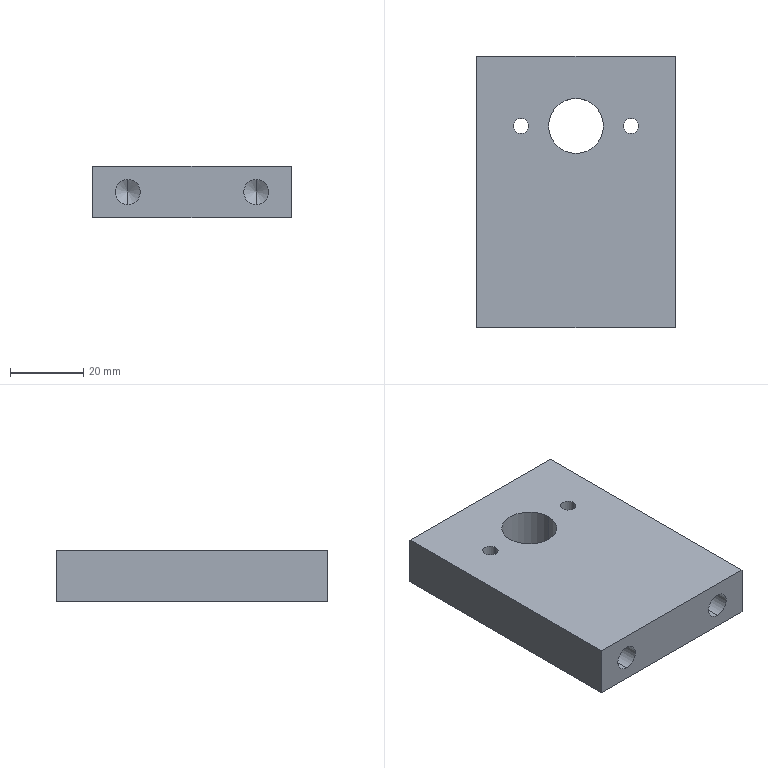Part | STEP file | PN_0065 (support block) | 1 solid | 20 faces | box 54 x 74 x 14 mm | volume 51598 mm3 | cylinder 10 | plane 6 | cone 4 | commonest cylinder face diameters 4.2 x4 6.8 x4 15 x2
STEP:
#1=CARTESIAN_POINT('',(0.,0.,0.));
#2=DIRECTION('',(0.,0.,1.));
#3=DIRECTION('',(1.,0.,0.));
#4=AXIS2_PLACEMENT_3D('',#1,#2,#3);
#5=CARTESIAN_POINT('',(-12.9,55.,-7.));
#6=VERTEX_POINT('',#5);
#7=CARTESIAN_POINT('',(-12.9,55.,7.));
#8=VERTEX_POINT('',#7);
#9=CARTESIAN_POINT('',(-12.9,55.,7.));
#10=DIRECTION('',(0.,0.,1.));
#11=VECTOR('',#10,1.);
#12=LINE('',#9,#11);
#13=CARTESIAN_POINT('',(-15.,55.,7.));
#14=DIRECTION('',(0.,0.,1.));
#15=DIRECTION('',(1.,0.,0.));
#16=AXIS2_PLACEMENT_3D('',#13,#14,#15);
#17=CYLINDRICAL_SURFACE('',#16,2.1);
#18=CARTESIAN_POINT('',(6.283,0.));
#19=DIRECTION('',(0.,1.));
#20=VECTOR('',#19,1.);
#21=LINE('',#18,#20);
#22=(GEOMETRIC_REPRESENTATION_CONTEXT(2)PARAMETRIC_REPRESENTATION_CONTEXT()REPRESENTATION_CONTEXT('',''));
#23=DEFINITIONAL_REPRESENTATION('',(#21),#22);
#24=PCURVE('',#17,#23);
#25=CARTESIAN_POINT('',(-15.,55.,7.));
#26=DIRECTION('',(0.,0.,1.));
#27=DIRECTION('',(1.,0.,0.));
#28=AXIS2_PLACEMENT_3D('',#25,#26,#27);
#29=CYLINDRICAL_SURFACE('',#28,2.1);
#30=CARTESIAN_POINT('',(0.,0.));
#31=DIRECTION('',(0.,1.));
#32=VECTOR('',#31,1.);
#33=LINE('',#30,#32);
#34=(GEOMETRIC_REPRESENTATION_CONTEXT(2)PARAMETRIC_REPRESENTATION_CONTEXT()REPRESENTATION_CONTEXT('',''));
#35=DEFINITIONAL_REPRESENTATION('',(#33),#34);
#36=PCURVE('',#29,#35);
#37=SURFACE_CURVE('',#12,(#24,#36),.PCURVE_S1.);
#38=EDGE_CURVE('',#6,#8,#37,.T.);
#39=ORIENTED_EDGE('',*,*,#38,.T.);
#40=CARTESIAN_POINT('',(-17.1,55.,7.));
#41=VERTEX_POINT('',#40);
#42=CARTESIAN_POINT('',(-15.,55.,7.));
#43=DIRECTION('',(0.,0.,1.));
#44=DIRECTION('',(1.,0.,0.));
#45=AXIS2_PLACEMENT_3D('',#42,#43,#44);
#46=CIRCLE('',#45,2.1);
#47=CARTESIAN_POINT('',(0.,0.));
#48=DIRECTION('',(1.,0.));
#49=VECTOR('',#48,1.);
#50=LINE('',#47,#49);
#51=(GEOMETRIC_REPRESENTATION_CONTEXT(2)PARAMETRIC_REPRESENTATION_CONTEXT()REPRESENTATION_CONTEXT('',''));
#52=DEFINITIONAL_REPRESENTATION('',(#50),#51);
#53=PCURVE('',#17,#52);
#54=CARTESIAN_POINT('',(0.,0.,7.));
#55=DIRECTION('',(0.,0.,-1.));
#56=DIRECTION('',(-1.,0.,0.));
#57=AXIS2_PLACEMENT_3D('',#54,#55,#56);
#58=PLANE('',#57);
#59=CARTESIAN_POINT('',(12.9,55.));
#60=CARTESIAN_POINT('',(12.9,58.637));
#61=CARTESIAN_POINT('',(16.05,56.819));
#62=CARTESIAN_POINT('',(19.2,55.));
#63=CARTESIAN_POINT('',(16.05,53.181));
#64=CARTESIAN_POINT('',(12.9,51.363));
#65=CARTESIAN_POINT('',(12.9,55.));
#66=(BOUNDED_CURVE()B_SPLINE_CURVE(2,(#59,#60,#61,#62,#63,#64,#65),.UNSPECIFIED.,.T.,.F.)B_SPLINE_CURVE_WITH_KNOTS((1,2,2,2,2,1),(-2.094,0.,2.094,4.189,6.283,8.378),.UNSPECIFIED.)CURVE()GEOMETRIC_REPRESENTATION_ITEM()RATIONAL_B_SPLINE_CURVE((1.,0.5,1.,0.5,1.,0.5,1.))REPRESENTATION_ITEM(''));
#67=(GEOMETRIC_REPRESENTATION_CONTEXT(2)PARAMETRIC_REPRESENTATION_CONTEXT()REPRESENTATION_CONTEXT('',''));
#68=DEFINITIONAL_REPRESENTATION('',(#66),#67);
#69=PCURVE('',#58,#68);
#70=SURFACE_CURVE('',#46,(#53,#69),.PCURVE_S1.);
#71=EDGE_CURVE('',#41,#8,#70,.T.);
#72=ORIENTED_EDGE('',*,*,#71,.F.);
#73=CARTESIAN_POINT('',(-17.1,55.,-7.));
#74=VERTEX_POINT('',#73);
#75=CARTESIAN_POINT('',(-17.1,55.,7.));
#76=DIRECTION('',(0.,0.,1.));
#77=VECTOR('',#76,1.);
#78=LINE('',#75,#77);
#79=CARTESIAN_POINT('',(3.142,0.));
#80=DIRECTION('',(0.,1.));
#81=VECTOR('',#80,1.);
#82=LINE('',#79,#81);
#83=(GEOMETRIC_REPRESENTATION_CONTEXT(2)PARAMETRIC_REPRESENTATION_CONTEXT()REPRESENTATION_CONTEXT('',''));
#84=DEFINITIONAL_REPRESENTATION('',(#82),#83);
#85=PCURVE('',#17,#84);
#86=CARTESIAN_POINT('',(3.142,0.));
#87=DIRECTION('',(0.,1.));
#88=VECTOR('',#87,1.);
#89=LINE('',#86,#88);
#90=(GEOMETRIC_REPRESENTATION_CONTEXT(2)PARAMETRIC_REPRESENTATION_CONTEXT()REPRESENTATION_CONTEXT('',''));
#91=DEFINITIONAL_REPRESENTATION('',(#89),#90);
#92=PCURVE('',#29,#91);
#93=SURFACE_CURVE('',#78,(#85,#92),.PCURVE_S1.);
#94=EDGE_CURVE('',#74,#41,#93,.T.);
#95=ORIENTED_EDGE('',*,*,#94,.F.);
#96=CARTESIAN_POINT('',(-15.,55.,-7.));
#97=DIRECTION('',(0.,0.,1.));
#98=DIRECTION('',(1.,0.,0.));
#99=AXIS2_PLACEMENT_3D('',#96,#97,#98);
#100=CIRCLE('',#99,2.1);
#101=CARTESIAN_POINT('',(0.,-14.));
#102=DIRECTION('',(1.,0.));
#103=VECTOR('',#102,1.);
#104=LINE('',#101,#103);
#105=(GEOMETRIC_REPRESENTATION_CONTEXT(2)PARAMETRIC_REPRESENTATION_CONTEXT()REPRESENTATION_CONTEXT('',''));
#106=DEFINITIONAL_REPRESENTATION('',(#104),#105);
#107=PCURVE('',#17,#106);
#108=CARTESIAN_POINT('',(0.,0.,-7.));
#109=DIRECTION('',(0.,0.,-1.));
#110=DIRECTION('',(-1.,0.,0.));
#111=AXIS2_PLACEMENT_3D('',#108,#109,#110);
#112=PLANE('',#111);
#113=CARTESIAN_POINT('',(12.9,55.));
#114=CARTESIAN_POINT('',(12.9,58.637));
#115=CARTESIAN_POINT('',(16.05,56.819));
#116=CARTESIAN_POINT('',(19.2,55.));
#117=CARTESIAN_POINT('',(16.05,53.181));
#118=CARTESIAN_POINT('',(12.9,51.363));
#119=CARTESIAN_POINT('',(12.9,55.));
#120=(BOUNDED_CURVE()B_SPLINE_CURVE(2,(#113,#114,#115,#116,#117,#118,#119),.UNSPECIFIED.,.T.,.F.)B_SPLINE_CURVE_WITH_KNOTS((1,2,2,2,2,1),(-2.094,0.,2.094,4.189,6.283,8.378),.UNSPECIFIED.)CURVE()GEOMETRIC_REPRESENTATION_ITEM()RATIONAL_B_SPLINE_CURVE((1.,0.5,1.,0.5,1.,0.5,1.))REPRESENTATION_ITEM(''));
#121=(GEOMETRIC_REPRESENTATION_CONTEXT(2)PARAMETRIC_REPRESENTATION_CONTEXT()REPRESENTATION_CONTEXT('',''));
#122=DEFINITIONAL_REPRESENTATION('',(#120),#121);
#123=PCURVE('',#112,#122);
#124=SURFACE_CURVE('',#100,(#107,#123),.PCURVE_S1.);
#125=EDGE_CURVE('',#74,#6,#124,.T.);
#126=ORIENTED_EDGE('',*,*,#125,.T.);
#127=EDGE_LOOP('',(#39,#72,#95,#126));
#128=FACE_BOUND('',#127,.F.);
#129=ADVANCED_FACE('',(#128),#17,.F.);
#130=CARTESIAN_POINT('',(17.1,55.,-7.));
#131=VERTEX_POINT('',#130);
#132=CARTESIAN_POINT('',(17.1,55.,7.));
#133=VERTEX_POINT('',#132);
#134=CARTESIAN_POINT('',(17.1,55.,7.));
#135=DIRECTION('',(0.,0.,1.));
#136=VECTOR('',#135,1.);
#137=LINE('',#134,#136);
#138=CARTESIAN_POINT('',(15.,55.,7.));
#139=DIRECTION('',(0.,0.,1.));
#140=DIRECTION('',(1.,0.,0.));
#141=AXIS2_PLACEMENT_3D('',#138,#139,#140);
#142=CYLINDRICAL_SURFACE('',#141,2.1);
#143=CARTESIAN_POINT('',(6.283,0.));
#144=DIRECTION('',(0.,1.));
#145=VECTOR('',#144,1.);
#146=LINE('',#143,#145);
#147=(GEOMETRIC_REPRESENTATION_CONTEXT(2)PARAMETRIC_REPRESENTATION_CONTEXT()REPRESENTATION_CONTEXT('',''));
#148=DEFINITIONAL_REPRESENTATION('',(#146),#147);
#149=PCURVE('',#142,#148);
#150=CARTESIAN_POINT('',(15.,55.,7.));
#151=DIRECTION('',(0.,0.,1.));
#152=DIRECTION('',(1.,0.,0.));
#153=AXIS2_PLACEMENT_3D('',#150,#151,#152);
#154=CYLINDRICAL_SURFACE('',#153,2.1);
#155=CARTESIAN_POINT('',(0.,0.));
#156=DIRECTION('',(0.,1.));
#157=VECTOR('',#156,1.);
#158=LINE('',#155,#157);
#159=(GEOMETRIC_REPRESENTATION_CONTEXT(2)PARAMETRIC_REPRESENTATION_CONTEXT()REPRESENTATION_CONTEXT('',''));
#160=DEFINITIONAL_REPRESENTATION('',(#158),#159);
#161=PCURVE('',#154,#160);
#162=SURFACE_CURVE('',#137,(#149,#161),.PCURVE_S1.);
#163=EDGE_CURVE('',#131,#133,#162,.T.);
#164=ORIENTED_EDGE('',*,*,#163,.T.);
#165=CARTESIAN_POINT('',(12.9,55.,7.));
#166=VERTEX_POINT('',#165);
#167=CARTESIAN_POINT('',(15.,55.,7.));
#168=DIRECTION('',(0.,0.,1.));
#169=DIRECTION('',(1.,0.,0.));
#170=AXIS2_PLACEMENT_3D('',#167,#168,#169);
#171=CIRCLE('',#170,2.1);
#172=CARTESIAN_POINT('',(0.,0.));
#173=DIRECTION('',(1.,0.));
#174=VECTOR('',#173,1.);
#175=LINE('',#172,#174);
#176=(GEOMETRIC_REPRESENTATION_CONTEXT(2)PARAMETRIC_REPRESENTATION_CONTEXT()REPRESENTATION_CONTEXT('',''));
#177=DEFINITIONAL_REPRESENTATION('',(#175),#176);
#178=PCURVE('',#142,#177);
#179=CARTESIAN_POINT('',(-17.1,55.));
#180=CARTESIAN_POINT('',(-17.1,58.637));
#181=CARTESIAN_POINT('',(-13.95,56.819));
#182=CARTESIAN_POINT('',(-10.8,55.));
#183=CARTESIAN_POINT('',(-13.95,53.181));
#184=CARTESIAN_POINT('',(-17.1,51.363));
#185=CARTESIAN_POINT('',(-17.1,55.));
#186=(BOUNDED_CURVE()B_SPLINE_CURVE(2,(#179,#180,#181,#182,#183,#184,#185),.UNSPECIFIED.,.T.,.F.)B_SPLINE_CURVE_WITH_KNOTS((1,2,2,2,2,1),(-2.094,0.,2.094,4.189,6.283,8.378),.UNSPECIFIED.)CURVE()GEOMETRIC_REPRESENTATION_ITEM()RATIONAL_B_SPLINE_CURVE((1.,0.5,1.,0.5,1.,0.5,1.))REPRESENTATION_ITEM(''));
#187=(GEOMETRIC_REPRESENTATION_CONTEXT(2)PARAMETRIC_REPRESENTATION_CONTEXT()REPRESENTATION_CONTEXT('',''));
#188=DEFINITIONAL_REPRESENTATION('',(#186),#187);
#189=PCURVE('',#58,#188);
#190=SURFACE_CURVE('',#171,(#178,#189),.PCURVE_S1.);
#191=EDGE_CURVE('',#166,#133,#190,.T.);
#192=ORIENTED_EDGE('',*,*,#191,.F.);
#193=CARTESIAN_POINT('',(12.9,55.,-7.));
#194=VERTEX_POINT('',#193);
#195=CARTESIAN_POINT('',(12.9,55.,7.));
#196=DIRECTION('',(0.,0.,1.));
#197=VECTOR('',#196,1.);
#198=LINE('',#195,#197);
#199=CARTESIAN_POINT('',(3.142,0.));
#200=DIRECTION('',(0.,1.));
#201=VECTOR('',#200,1.);
#202=LINE('',#199,#201);
#203=(GEOMETRIC_REPRESENTATION_CONTEXT(2)PARAMETRIC_REPRESENTATION_CONTEXT()REPRESENTATION_CONTEXT('',''));
#204=DEFINITIONAL_REPRESENTATION('',(#202),#203);
#205=PCURVE('',#142,#204);
#206=CARTESIAN_POINT('',(3.142,0.));
#207=DIRECTION('',(0.,1.));
#208=VECTOR('',#207,1.);
#209=LINE('',#206,#208);
#210=(GEOMETRIC_REPRESENTATION_CONTEXT(2)PARAMETRIC_REPRESENTATION_CONTEXT()REPRESENTATION_CONTEXT('',''));
#211=DEFINITIONAL_REPRESENTATION('',(#209),#210);
#212=PCURVE('',#154,#211);
#213=SURFACE_CURVE('',#198,(#205,#212),.PCURVE_S1.);
#214=EDGE_CURVE('',#194,#166,#213,.T.);
#215=ORIENTED_EDGE('',*,*,#214,.F.);
#216=CARTESIAN_POINT('',(15.,55.,-7.));
#217=DIRECTION('',(0.,0.,1.));
#218=DIRECTION('',(1.,0.,0.));
#219=AXIS2_PLACEMENT_3D('',#216,#217,#218);
#220=CIRCLE('',#219,2.1);
#221=CARTESIAN_POINT('',(0.,-14.));
#222=DIRECTION('',(1.,0.));
#223=VECTOR('',#222,1.);
#224=LINE('',#221,#223);
#225=(GEOMETRIC_REPRESENTATION_CONTEXT(2)PARAMETRIC_REPRESENTATION_CONTEXT()REPRESENTATION_CONTEXT('',''));
#226=DEFINITIONAL_REPRESENTATION('',(#224),#225);
#227=PCURVE('',#142,#226);
#228=CARTESIAN_POINT('',(-17.1,55.));
#229=CARTESIAN_POINT('',(-17.1,58.637));
#230=CARTESIAN_POINT('',(-13.95,56.819));
#231=CARTESIAN_POINT('',(-10.8,55.));
#232=CARTESIAN_POINT('',(-13.95,53.181));
#233=CARTESIAN_POINT('',(-17.1,51.363));
#234=CARTESIAN_POINT('',(-17.1,55.));
#235=(BOUNDED_CURVE()B_SPLINE_CURVE(2,(#228,#229,#230,#231,#232,#233,#234),.UNSPECIFIED.,.T.,.F.)B_SPLINE_CURVE_WITH_KNOTS((1,2,2,2,2,1),(-2.094,0.,2.094,4.189,6.283,8.378),.UNSPECIFIED.)CURVE()GEOMETRIC_REPRESENTATION_ITEM()RATIONAL_B_SPLINE_CURVE((1.,0.5,1.,0.5,1.,0.5,1.))REPRESENTATION_ITEM(''));
#236=(GEOMETRIC_REPRESENTATION_CONTEXT(2)PARAMETRIC_REPRESENTATION_CONTEXT()REPRESENTATION_CONTEXT('',''));
#237=DEFINITIONAL_REPRESENTATION('',(#235),#236);
#238=PCURVE('',#112,#237);
#239=SURFACE_CURVE('',#220,(#227,#238),.PCURVE_S1.);
#240=EDGE_CURVE('',#194,#131,#239,.T.);
#241=ORIENTED_EDGE('',*,*,#240,.T.);
#242=EDGE_LOOP('',(#164,#192,#215,#241));
#243=FACE_BOUND('',#242,.F.);
#244=ADVANCED_FACE('',(#243),#142,.F.);
#245=CARTESIAN_POINT('',(-7.5,55.,7.));
#246=VERTEX_POINT('',#245);
#247=CARTESIAN_POINT('',(-7.5,55.,-7.));
#248=VERTEX_POINT('',#247);
#249=CARTESIAN_POINT('',(-7.5,55.,7.));
#250=DIRECTION('',(0.,0.,-1.));
#251=VECTOR('',#250,1.);
#252=LINE('',#249,#251);
#253=CARTESIAN_POINT('',(0.,55.,7.));
#254=DIRECTION('',(0.,0.,-1.));
#255=DIRECTION('',(-1.,0.,0.));
#256=AXIS2_PLACEMENT_3D('',#253,#254,#255);
#257=CYLINDRICAL_SURFACE('',#256,7.5);
#258=CARTESIAN_POINT('',(6.283,0.));
#259=DIRECTION('',(0.,1.));
#260=VECTOR('',#259,1.);
#261=LINE('',#258,#260);
#262=(GEOMETRIC_REPRESENTATION_CONTEXT(2)PARAMETRIC_REPRESENTATION_CONTEXT()REPRESENTATION_CONTEXT('',''));
#263=DEFINITIONAL_REPRESENTATION('',(#261),#262);
#264=PCURVE('',#257,#263);
#265=CARTESIAN_POINT('',(0.,55.,7.));
#266=DIRECTION('',(0.,0.,-1.));
#267=DIRECTION('',(-1.,0.,0.));
#268=AXIS2_PLACEMENT_3D('',#265,#266,#267);
#269=CYLINDRICAL_SURFACE('',#268,7.5);
#270=CARTESIAN_POINT('',(0.,0.));
#271=DIRECTION('',(0.,1.));
#272=VECTOR('',#271,1.);
#273=LINE('',#270,#272);
#274=(GEOMETRIC_REPRESENTATION_CONTEXT(2)PARAMETRIC_REPRESENTATION_CONTEXT()REPRESENTATION_CONTEXT('',''));
#275=DEFINITIONAL_REPRESENTATION('',(#273),#274);
#276=PCURVE('',#269,#275);
#277=SURFACE_CURVE('',#252,(#264,#276),.PCURVE_S1.);
#278=EDGE_CURVE('',#246,#248,#277,.T.);
#279=ORIENTED_EDGE('',*,*,#278,.T.);
#280=CARTESIAN_POINT('',(7.5,55.,-7.));
#281=VERTEX_POINT('',#280);
#282=CARTESIAN_POINT('',(0.,55.,-7.));
#283=DIRECTION('',(0.,0.,-1.));
#284=DIRECTION('',(-1.,0.,0.));
#285=AXIS2_PLACEMENT_3D('',#282,#283,#284);
#286=CIRCLE('',#285,7.5);
#287=CARTESIAN_POINT('',(0.,14.));
#288=DIRECTION('',(1.,0.));
#289=VECTOR('',#288,1.);
#290=LINE('',#287,#289);
#291=(GEOMETRIC_REPRESENTATION_CONTEXT(2)PARAMETRIC_REPRESENTATION_CONTEXT()REPRESENTATION_CONTEXT('',''));
#292=DEFINITIONAL_REPRESENTATION('',(#290),#291);
#293=PCURVE('',#257,#292);
#294=CARTESIAN_POINT('',(0.,55.));
#295=DIRECTION('',(1.,0.));
#296=AXIS2_PLACEMENT_2D('',#294,#295);
#297=CIRCLE('',#296,7.5);
#298=(GEOMETRIC_REPRESENTATION_CONTEXT(2)PARAMETRIC_REPRESENTATION_CONTEXT()REPRESENTATION_CONTEXT('',''));
#299=DEFINITIONAL_REPRESENTATION('',(#297),#298);
#300=PCURVE('',#112,#299);
#301=SURFACE_CURVE('',#286,(#293,#300),.PCURVE_S1.);
#302=EDGE_CURVE('',#281,#248,#301,.T.);
#303=ORIENTED_EDGE('',*,*,#302,.F.);
#304=CARTESIAN_POINT('',(7.5,55.,7.));
#305=VERTEX_POINT('',#304);
#306=CARTESIAN_POINT('',(7.5,55.,7.));
#307=DIRECTION('',(0.,0.,-1.));
#308=VECTOR('',#307,1.);
#309=LINE('',#306,#308);
#310=CARTESIAN_POINT('',(3.142,0.));
#311=DIRECTION('',(0.,1.));
#312=VECTOR('',#311,1.);
#313=LINE('',#310,#312);
#314=(GEOMETRIC_REPRESENTATION_CONTEXT(2)PARAMETRIC_REPRESENTATION_CONTEXT()REPRESENTATION_CONTEXT('',''));
#315=DEFINITIONAL_REPRESENTATION('',(#313),#314);
#316=PCURVE('',#257,#315);
#317=CARTESIAN_POINT('',(3.142,0.));
#318=DIRECTION('',(0.,1.));
#319=VECTOR('',#318,1.);
#320=LINE('',#317,#319);
#321=(GEOMETRIC_REPRESENTATION_CONTEXT(2)PARAMETRIC_REPRESENTATION_CONTEXT()REPRESENTATION_CONTEXT('',''));
#322=DEFINITIONAL_REPRESENTATION('',(#320),#321);
#323=PCURVE('',#269,#322);
#324=SURFACE_CURVE('',#309,(#316,#323),.PCURVE_S1.);
#325=EDGE_CURVE('',#305,#281,#324,.T.);
#326=ORIENTED_EDGE('',*,*,#325,.F.);
#327=CARTESIAN_POINT('',(0.,55.,7.));
#328=DIRECTION('',(0.,0.,-1.));
#329=DIRECTION('',(-1.,0.,0.));
#330=AXIS2_PLACEMENT_3D('',#327,#328,#329);
#331=CIRCLE('',#330,7.5);
#332=CARTESIAN_POINT('',(0.,0.));
#333=DIRECTION('',(1.,0.));
#334=VECTOR('',#333,1.);
#335=LINE('',#332,#334);
#336=(GEOMETRIC_REPRESENTATION_CONTEXT(2)PARAMETRIC_REPRESENTATION_CONTEXT()REPRESENTATION_CONTEXT('',''));
#337=DEFINITIONAL_REPRESENTATION('',(#335),#336);
#338=PCURVE('',#257,#337);
#339=CARTESIAN_POINT('',(0.,55.));
#340=DIRECTION('',(1.,0.));
#341=AXIS2_PLACEMENT_2D('',#339,#340);
#342=CIRCLE('',#341,7.5);
#343=(GEOMETRIC_REPRESENTATION_CONTEXT(2)PARAMETRIC_REPRESENTATION_CONTEXT()REPRESENTATION_CONTEXT('',''));
#344=DEFINITIONAL_REPRESENTATION('',(#342),#343);
#345=PCURVE('',#58,#344);
#346=SURFACE_CURVE('',#331,(#338,#345),.PCURVE_S1.);
#347=EDGE_CURVE('',#305,#246,#346,.T.);
#348=ORIENTED_EDGE('',*,*,#347,.T.);
#349=EDGE_LOOP('',(#279,#303,#326,#348));
#350=FACE_BOUND('',#349,.F.);
#351=ADVANCED_FACE('',(#350),#257,.F.);
#352=CARTESIAN_POINT('',(-17.5,19.75,-3.4));
#353=VERTEX_POINT('',#352);
#354=CARTESIAN_POINT('',(-17.5,0.,-3.4));
#355=VERTEX_POINT('',#354);
#356=CARTESIAN_POINT('',(-17.5,0.,-3.4));
#357=DIRECTION('',(0.,-1.,0.));
#358=VECTOR('',#357,1.);
#359=LINE('',#356,#358);
#360=CARTESIAN_POINT('',(-17.5,0.,0.));
#361=DIRECTION('',(0.,-1.,0.));
#362=DIRECTION('',(0.,0.,-1.));
#363=AXIS2_PLACEMENT_3D('',#360,#361,#362);
#364=CYLINDRICAL_SURFACE('',#363,3.4);
#365=CARTESIAN_POINT('',(6.283,0.));
#366=DIRECTION('',(0.,1.));
#367=VECTOR('',#366,1.);
#368=LINE('',#365,#367);
#369=(GEOMETRIC_REPRESENTATION_CONTEXT(2)PARAMETRIC_REPRESENTATION_CONTEXT()REPRESENTATION_CONTEXT('',''));
#370=DEFINITIONAL_REPRESENTATION('',(#368),#369);
#371=PCURVE('',#364,#370);
#372=CARTESIAN_POINT('',(-17.5,0.,0.));
#373=DIRECTION('',(0.,-1.,0.));
#374=DIRECTION('',(0.,0.,-1.));
#375=AXIS2_PLACEMENT_3D('',#372,#373,#374);
#376=CYLINDRICAL_SURFACE('',#375,3.4);
#377=CARTESIAN_POINT('',(0.,0.));
#378=DIRECTION('',(0.,1.));
#379=VECTOR('',#378,1.);
#380=LINE('',#377,#379);
#381=(GEOMETRIC_REPRESENTATION_CONTEXT(2)PARAMETRIC_REPRESENTATION_CONTEXT()REPRESENTATION_CONTEXT('',''));
#382=DEFINITIONAL_REPRESENTATION('',(#380),#381);
#383=PCURVE('',#376,#382);
#384=SURFACE_CURVE('',#359,(#371,#383),.PCURVE_S1.);
#385=EDGE_CURVE('',#353,#355,#384,.T.);
#386=ORIENTED_EDGE('',*,*,#385,.T.);
#387=CARTESIAN_POINT('',(-17.5,0.,3.4));
#388=VERTEX_POINT('',#387);
#389=CARTESIAN_POINT('',(-17.5,0.,0.));
#390=DIRECTION('',(0.,-1.,0.));
#391=DIRECTION('',(0.,0.,-1.));
#392=AXIS2_PLACEMENT_3D('',#389,#390,#391);
#393=CIRCLE('',#392,3.4);
#394=CARTESIAN_POINT('',(0.,0.));
#395=DIRECTION('',(1.,0.));
#396=VECTOR('',#395,1.);
#397=LINE('',#394,#396);
#398=(GEOMETRIC_REPRESENTATION_CONTEXT(2)PARAMETRIC_REPRESENTATION_CONTEXT()REPRESENTATION_CONTEXT('',''));
#399=DEFINITIONAL_REPRESENTATION('',(#397),#398);
#400=PCURVE('',#364,#399);
#401=CARTESIAN_POINT('',(-27.,0.,7.));
#402=DIRECTION('',(0.,1.,0.));
#403=DIRECTION('',(0.,0.,1.));
#404=AXIS2_PLACEMENT_3D('',#401,#402,#403);
#405=PLANE('',#404);
#406=CARTESIAN_POINT('',(-10.4,9.5));
#407=CARTESIAN_POINT('',(-10.4,15.389));
#408=CARTESIAN_POINT('',(-5.3,12.444));
#409=CARTESIAN_POINT('',(-0.2,9.5));
#410=CARTESIAN_POINT('',(-5.3,6.556));
#411=CARTESIAN_POINT('',(-10.4,3.611));
#412=CARTESIAN_POINT('',(-10.4,9.5));
#413=(BOUNDED_CURVE()B_SPLINE_CURVE(2,(#406,#407,#408,#409,#410,#411,#412),.UNSPECIFIED.,.T.,.F.)B_SPLINE_CURVE_WITH_KNOTS((1,2,2,2,2,1),(-2.094,0.,2.094,4.189,6.283,8.378),.UNSPECIFIED.)CURVE()GEOMETRIC_REPRESENTATION_ITEM()RATIONAL_B_SPLINE_CURVE((1.,0.5,1.,0.5,1.,0.5,1.))REPRESENTATION_ITEM(''));
#414=(GEOMETRIC_REPRESENTATION_CONTEXT(2)PARAMETRIC_REPRESENTATION_CONTEXT()REPRESENTATION_CONTEXT('',''));
#415=DEFINITIONAL_REPRESENTATION('',(#413),#414);
#416=PCURVE('',#405,#415);
#417=SURFACE_CURVE('',#393,(#400,#416),.PCURVE_S1.);
#418=EDGE_CURVE('',#388,#355,#417,.T.);
#419=ORIENTED_EDGE('',*,*,#418,.F.);
#420=CARTESIAN_POINT('',(-17.5,19.75,3.4));
#421=VERTEX_POINT('',#420);
#422=CARTESIAN_POINT('',(-17.5,0.,3.4));
#423=DIRECTION('',(0.,-1.,0.));
#424=VECTOR('',#423,1.);
#425=LINE('',#422,#424);
#426=CARTESIAN_POINT('',(3.142,0.));
#427=DIRECTION('',(0.,1.));
#428=VECTOR('',#427,1.);
#429=LINE('',#426,#428);
#430=(GEOMETRIC_REPRESENTATION_CONTEXT(2)PARAMETRIC_REPRESENTATION_CONTEXT()REPRESENTATION_CONTEXT('',''));
#431=DEFINITIONAL_REPRESENTATION('',(#429),#430);
#432=PCURVE('',#364,#431);
#433=CARTESIAN_POINT('',(3.142,0.));
#434=DIRECTION('',(0.,1.));
#435=VECTOR('',#434,1.);
#436=LINE('',#433,#435);
#437=(GEOMETRIC_REPRESENTATION_CONTEXT(2)PARAMETRIC_REPRESENTATION_CONTEXT()REPRESENTATION_CONTEXT('',''));
#438=DEFINITIONAL_REPRESENTATION('',(#436),#437);
#439=PCURVE('',#376,#438);
#440=SURFACE_CURVE('',#425,(#432,#439),.PCURVE_S1.);
#441=EDGE_CURVE('',#421,#388,#440,.T.);
#442=ORIENTED_EDGE('',*,*,#441,.F.);
#443=CARTESIAN_POINT('',(-17.5,19.75,0.));
#444=DIRECTION('',(0.,-1.,0.));
#445=DIRECTION('',(0.,0.,-1.));
#446=AXIS2_PLACEMENT_3D('',#443,#444,#445);
#447=CIRCLE('',#446,3.4);
#448=CARTESIAN_POINT('',(0.,-19.75));
#449=DIRECTION('',(1.,0.));
#450=VECTOR('',#449,1.);
#451=LINE('',#448,#450);
#452=(GEOMETRIC_REPRESENTATION_CONTEXT(2)PARAMETRIC_REPRESENTATION_CONTEXT()REPRESENTATION_CONTEXT('',''));
#453=DEFINITIONAL_REPRESENTATION('',(#451),#452);
#454=PCURVE('',#364,#453);
#455=CARTESIAN_POINT('',(-17.5,19.75,0.));
#456=DIRECTION('',(0.,-1.,0.));
#457=DIRECTION('',(0.,0.,-1.));
#458=AXIS2_PLACEMENT_3D('',#455,#456,#457);
#459=CONICAL_SURFACE('',#458,3.4,1.03);
#460=CARTESIAN_POINT('',(0.,0.));
#461=DIRECTION('',(1.,0.));
#462=VECTOR('',#461,1.);
#463=LINE('',#460,#462);
#464=(GEOMETRIC_REPRESENTATION_CONTEXT(2)PARAMETRIC_REPRESENTATION_CONTEXT()REPRESENTATION_CONTEXT('',''));
#465=DEFINITIONAL_REPRESENTATION('',(#463),#464);
#466=PCURVE('',#459,#465);
#467=SURFACE_CURVE('',#447,(#454,#466),.PCURVE_S1.);
#468=EDGE_CURVE('',#421,#353,#467,.T.);
#469=ORIENTED_EDGE('',*,*,#468,.T.);
#470=EDGE_LOOP('',(#386,#419,#442,#469));
#471=FACE_BOUND('',#470,.F.);
#472=ADVANCED_FACE('',(#471),#364,.F.);
#473=ORIENTED_EDGE('',*,*,#468,.F.);
#474=CARTESIAN_POINT('',(-17.5,21.793,0.));
#475=VERTEX_POINT('',#474);
#476=CARTESIAN_POINT('',(-17.5,19.75,3.4));
#477=DIRECTION('',(0.,-0.515,0.8572));
#478=VECTOR('',#477,1.);
#479=LINE('',#476,#478);
#480=CARTESIAN_POINT('',(3.142,0.));
#481=DIRECTION('',(0.,1.));
#482=VECTOR('',#481,1.);
#483=LINE('',#480,#482);
#484=(GEOMETRIC_REPRESENTATION_CONTEXT(2)PARAMETRIC_REPRESENTATION_CONTEXT()REPRESENTATION_CONTEXT('',''));
#485=DEFINITIONAL_REPRESENTATION('',(#483),#484);
#486=PCURVE('',#459,#485);
#487=CARTESIAN_POINT('',(-17.5,19.75,0.));
#488=DIRECTION('',(0.,-1.,0.));
#489=DIRECTION('',(0.,0.,-1.));
#490=AXIS2_PLACEMENT_3D('',#487,#488,#489);
#491=CONICAL_SURFACE('',#490,3.4,1.03);
#492=CARTESIAN_POINT('',(3.142,0.));
#493=DIRECTION('',(0.,1.));
#494=VECTOR('',#493,1.);
#495=LINE('',#492,#494);
#496=(GEOMETRIC_REPRESENTATION_CONTEXT(2)PARAMETRIC_REPRESENTATION_CONTEXT()REPRESENTATION_CONTEXT('',''));
#497=DEFINITIONAL_REPRESENTATION('',(#495),#496);
#498=PCURVE('',#491,#497);
#499=SURFACE_CURVE('',#479,(#486,#498),.PCURVE_S1.);
#500=EDGE_CURVE('',#475,#421,#499,.T.);
#501=ORIENTED_EDGE('',*,*,#500,.F.);
#502=CARTESIAN_POINT('',(-17.5,19.75,-3.4));
#503=DIRECTION('',(0.,-0.515,-0.8572));
#504=VECTOR('',#503,1.);
#505=LINE('',#502,#504);
#506=CARTESIAN_POINT('',(6.283,0.));
#507=DIRECTION('',(0.,1.));
#508=VECTOR('',#507,1.);
#509=LINE('',#506,#508);
#510=(GEOMETRIC_REPRESENTATION_CONTEXT(2)PARAMETRIC_REPRESENTATION_CONTEXT()REPRESENTATION_CONTEXT('',''));
#511=DEFINITIONAL_REPRESENTATION('',(#509),#510);
#512=PCURVE('',#459,#511);
#513=CARTESIAN_POINT('',(0.,0.));
#514=DIRECTION('',(0.,1.));
#515=VECTOR('',#514,1.);
#516=LINE('',#513,#515);
#517=(GEOMETRIC_REPRESENTATION_CONTEXT(2)PARAMETRIC_REPRESENTATION_CONTEXT()REPRESENTATION_CONTEXT('',''));
#518=DEFINITIONAL_REPRESENTATION('',(#516),#517);
#519=PCURVE('',#491,#518);
#520=SURFACE_CURVE('',#505,(#512,#519),.PCURVE_S1.);
#521=EDGE_CURVE('',#475,#353,#520,.T.);
#522=ORIENTED_EDGE('',*,*,#521,.T.);
#523=EDGE_LOOP('',(#473,#501,#522));
#524=FACE_BOUND('',#523,.F.);
#525=ADVANCED_FACE('',(#524),#459,.F.);
#526=CARTESIAN_POINT('',(17.5,19.75,-3.4));
#527=VERTEX_POINT('',#526);
#528=CARTESIAN_POINT('',(17.5,0.,-3.4));
#529=VERTEX_POINT('',#528);
#530=CARTESIAN_POINT('',(17.5,0.,-3.4));
#531=DIRECTION('',(0.,-1.,0.));
#532=VECTOR('',#531,1.);
#533=LINE('',#530,#532);
#534=CARTESIAN_POINT('',(17.5,0.,0.));
#535=DIRECTION('',(0.,-1.,0.));
#536=DIRECTION('',(0.,0.,-1.));
#537=AXIS2_PLACEMENT_3D('',#534,#535,#536);
#538=CYLINDRICAL_SURFACE('',#537,3.4);
#539=CARTESIAN_POINT('',(6.283,0.));
#540=DIRECTION('',(0.,1.));
#541=VECTOR('',#540,1.);
#542=LINE('',#539,#541);
#543=(GEOMETRIC_REPRESENTATION_CONTEXT(2)PARAMETRIC_REPRESENTATION_CONTEXT()REPRESENTATION_CONTEXT('',''));
#544=DEFINITIONAL_REPRESENTATION('',(#542),#543);
#545=PCURVE('',#538,#544);
#546=CARTESIAN_POINT('',(17.5,0.,0.));
#547=DIRECTION('',(0.,-1.,0.));
#548=DIRECTION('',(0.,0.,-1.));
#549=AXIS2_PLACEMENT_3D('',#546,#547,#548);
#550=CYLINDRICAL_SURFACE('',#549,3.4);
#551=CARTESIAN_POINT('',(0.,0.));
#552=DIRECTION('',(0.,1.));
#553=VECTOR('',#552,1.);
#554=LINE('',#551,#553);
#555=(GEOMETRIC_REPRESENTATION_CONTEXT(2)PARAMETRIC_REPRESENTATION_CONTEXT()REPRESENTATION_CONTEXT('',''));
#556=DEFINITIONAL_REPRESENTATION('',(#554),#555);
#557=PCURVE('',#550,#556);
#558=SURFACE_CURVE('',#533,(#545,#557),.PCURVE_S1.);
#559=EDGE_CURVE('',#527,#529,#558,.T.);
#560=ORIENTED_EDGE('',*,*,#559,.T.);
#561=CARTESIAN_POINT('',(17.5,0.,3.4));
#562=VERTEX_POINT('',#561);
#563=CARTESIAN_POINT('',(17.5,0.,0.));
#564=DIRECTION('',(0.,-1.,0.));
#565=DIRECTION('',(0.,0.,-1.));
#566=AXIS2_PLACEMENT_3D('',#563,#564,#565);
#567=CIRCLE('',#566,3.4);
#568=CARTESIAN_POINT('',(0.,0.));
#569=DIRECTION('',(1.,0.));
#570=VECTOR('',#569,1.);
#571=LINE('',#568,#570);
#572=(GEOMETRIC_REPRESENTATION_CONTEXT(2)PARAMETRIC_REPRESENTATION_CONTEXT()REPRESENTATION_CONTEXT('',''));
#573=DEFINITIONAL_REPRESENTATION('',(#571),#572);
#574=PCURVE('',#538,#573);
#575=CARTESIAN_POINT('',(-10.4,44.5));
#576=CARTESIAN_POINT('',(-10.4,50.389));
#577=CARTESIAN_POINT('',(-5.3,47.444));
#578=CARTESIAN_POINT('',(-0.2,44.5));
#579=CARTESIAN_POINT('',(-5.3,41.556));
#580=CARTESIAN_POINT('',(-10.4,38.611));
#581=CARTESIAN_POINT('',(-10.4,44.5));
#582=(BOUNDED_CURVE()B_SPLINE_CURVE(2,(#575,#576,#577,#578,#579,#580,#581),.UNSPECIFIED.,.T.,.F.)B_SPLINE_CURVE_WITH_KNOTS((1,2,2,2,2,1),(-2.094,0.,2.094,4.189,6.283,8.378),.UNSPECIFIED.)CURVE()GEOMETRIC_REPRESENTATION_ITEM()RATIONAL_B_SPLINE_CURVE((1.,0.5,1.,0.5,1.,0.5,1.))REPRESENTATION_ITEM(''));
#583=(GEOMETRIC_REPRESENTATION_CONTEXT(2)PARAMETRIC_REPRESENTATION_CONTEXT()REPRESENTATION_CONTEXT('',''));
#584=DEFINITIONAL_REPRESENTATION('',(#582),#583);
#585=PCURVE('',#405,#584);
#586=SURFACE_CURVE('',#567,(#574,#585),.PCURVE_S1.);
#587=EDGE_CURVE('',#562,#529,#586,.T.);
#588=ORIENTED_EDGE('',*,*,#587,.F.);
#589=CARTESIAN_POINT('',(17.5,19.75,3.4));
#590=VERTEX_POINT('',#589);
#591=CARTESIAN_POINT('',(17.5,0.,3.4));
#592=DIRECTION('',(0.,-1.,0.));
#593=VECTOR('',#592,1.);
#594=LINE('',#591,#593);
#595=CARTESIAN_POINT('',(3.142,0.));
#596=DIRECTION('',(0.,1.));
#597=VECTOR('',#596,1.);
#598=LINE('',#595,#597);
#599=(GEOMETRIC_REPRESENTATION_CONTEXT(2)PARAMETRIC_REPRESENTATION_CONTEXT()REPRESENTATION_CONTEXT('',''));
#600=DEFINITIONAL_REPRESENTATION('',(#598),#599);
#601=PCURVE('',#538,#600);
#602=CARTESIAN_POINT('',(3.142,0.));
#603=DIRECTION('',(0.,1.));
#604=VECTOR('',#603,1.);
#605=LINE('',#602,#604);
#606=(GEOMETRIC_REPRESENTATION_CONTEXT(2)PARAMETRIC_REPRESENTATION_CONTEXT()REPRESENTATION_CONTEXT('',''));
#607=DEFINITIONAL_REPRESENTATION('',(#605),#606);
#608=PCURVE('',#550,#607);
#609=SURFACE_CURVE('',#594,(#601,#608),.PCURVE_S1.);
#610=EDGE_CURVE('',#590,#562,#609,.T.);
#611=ORIENTED_EDGE('',*,*,#610,.F.);
#612=CARTESIAN_POINT('',(17.5,19.75,0.));
#613=DIRECTION('',(0.,-1.,0.));
#614=DIRECTION('',(0.,0.,-1.));
#615=AXIS2_PLACEMENT_3D('',#612,#613,#614);
#616=CIRCLE('',#615,3.4);
#617=CARTESIAN_POINT('',(0.,-19.75));
#618=DIRECTION('',(1.,0.));
#619=VECTOR('',#618,1.);
#620=LINE('',#617,#619);
#621=(GEOMETRIC_REPRESENTATION_CONTEXT(2)PARAMETRIC_REPRESENTATION_CONTEXT()REPRESENTATION_CONTEXT('',''));
#622=DEFINITIONAL_REPRESENTATION('',(#620),#621);
#623=PCURVE('',#538,#622);
#624=CARTESIAN_POINT('',(17.5,19.75,0.));
#625=DIRECTION('',(0.,-1.,0.));
#626=DIRECTION('',(0.,0.,-1.));
#627=AXIS2_PLACEMENT_3D('',#624,#625,#626);
#628=CONICAL_SURFACE('',#627,3.4,1.03);
#629=CARTESIAN_POINT('',(0.,0.));
#630=DIRECTION('',(1.,0.));
#631=VECTOR('',#630,1.);
#632=LINE('',#629,#631);
#633=(GEOMETRIC_REPRESENTATION_CONTEXT(2)PARAMETRIC_REPRESENTATION_CONTEXT()REPRESENTATION_CONTEXT('',''));
#634=DEFINITIONAL_REPRESENTATION('',(#632),#633);
#635=PCURVE('',#628,#634);
#636=SURFACE_CURVE('',#616,(#623,#635),.PCURVE_S1.);
#637=EDGE_CURVE('',#590,#527,#636,.T.);
#638=ORIENTED_EDGE('',*,*,#637,.T.);
#639=EDGE_LOOP('',(#560,#588,#611,#638));
#640=FACE_BOUND('',#639,.F.);
#641=ADVANCED_FACE('',(#640),#538,.F.);
#642=ORIENTED_EDGE('',*,*,#637,.F.);
#643=CARTESIAN_POINT('',(17.5,21.793,0.));
#644=VERTEX_POINT('',#643);
#645=CARTESIAN_POINT('',(17.5,19.75,3.4));
#646=DIRECTION('',(0.,-0.515,0.8572));
#647=VECTOR('',#646,1.);
#648=LINE('',#645,#647);
#649=CARTESIAN_POINT('',(3.142,0.));
#650=DIRECTION('',(0.,1.));
#651=VECTOR('',#650,1.);
#652=LINE('',#649,#651);
#653=(GEOMETRIC_REPRESENTATION_CONTEXT(2)PARAMETRIC_REPRESENTATION_CONTEXT()REPRESENTATION_CONTEXT('',''));
#654=DEFINITIONAL_REPRESENTATION('',(#652),#653);
#655=PCURVE('',#628,#654);
#656=CARTESIAN_POINT('',(17.5,19.75,0.));
#657=DIRECTION('',(0.,-1.,0.));
#658=DIRECTION('',(0.,0.,-1.));
#659=AXIS2_PLACEMENT_3D('',#656,#657,#658);
#660=CONICAL_SURFACE('',#659,3.4,1.03);
#661=CARTESIAN_POINT('',(3.142,0.));
#662=DIRECTION('',(0.,1.));
#663=VECTOR('',#662,1.);
#664=LINE('',#661,#663);
#665=(GEOMETRIC_REPRESENTATION_CONTEXT(2)PARAMETRIC_REPRESENTATION_CONTEXT()REPRESENTATION_CONTEXT('',''));
#666=DEFINITIONAL_REPRESENTATION('',(#664),#665);
#667=PCURVE('',#660,#666);
#668=SURFACE_CURVE('',#648,(#655,#667),.PCURVE_S1.);
#669=EDGE_CURVE('',#644,#590,#668,.T.);
#670=ORIENTED_EDGE('',*,*,#669,.F.);
#671=CARTESIAN_POINT('',(17.5,19.75,-3.4));
#672=DIRECTION('',(0.,-0.515,-0.8572));
#673=VECTOR('',#672,1.);
#674=LINE('',#671,#673);
#675=CARTESIAN_POINT('',(6.283,0.));
#676=DIRECTION('',(0.,1.));
#677=VECTOR('',#676,1.);
#678=LINE('',#675,#677);
#679=(GEOMETRIC_REPRESENTATION_CONTEXT(2)PARAMETRIC_REPRESENTATION_CONTEXT()REPRESENTATION_CONTEXT('',''));
#680=DEFINITIONAL_REPRESENTATION('',(#678),#679);
#681=PCURVE('',#628,#680);
#682=CARTESIAN_POINT('',(0.,0.));
#683=DIRECTION('',(0.,1.));
#684=VECTOR('',#683,1.);
#685=LINE('',#682,#684);
#686=(GEOMETRIC_REPRESENTATION_CONTEXT(2)PARAMETRIC_REPRESENTATION_CONTEXT()REPRESENTATION_CONTEXT('',''));
#687=DEFINITIONAL_REPRESENTATION('',(#685),#686);
#688=PCURVE('',#660,#687);
#689=SURFACE_CURVE('',#674,(#681,#688),.PCURVE_S1.);
#690=EDGE_CURVE('',#644,#527,#689,.T.);
#691=ORIENTED_EDGE('',*,*,#690,.T.);
#692=EDGE_LOOP('',(#642,#670,#691));
#693=FACE_BOUND('',#692,.F.);
#694=ADVANCED_FACE('',(#693),#628,.F.);
#695=CARTESIAN_POINT('',(-27.,74.,-7.));
#696=VERTEX_POINT('',#695);
#697=CARTESIAN_POINT('',(-27.,0.,-7.));
#698=VERTEX_POINT('',#697);
#699=CARTESIAN_POINT('',(-27.,0.,-7.));
#700=DIRECTION('',(0.,-1.,0.));
#701=VECTOR('',#700,1.);
#702=LINE('',#699,#701);
#703=CARTESIAN_POINT('',(-27.,0.,7.));
#704=DIRECTION('',(1.,0.,0.));
#705=DIRECTION('',(0.,0.,-1.));
#706=AXIS2_PLACEMENT_3D('',#703,#704,#705);
#707=PLANE('',#706);
#708=CARTESIAN_POINT('',(14.,0.));
#709=DIRECTION('',(0.,-1.));
#710=VECTOR('',#709,1.);
#711=LINE('',#708,#710);
#712=(GEOMETRIC_REPRESENTATION_CONTEXT(2)PARAMETRIC_REPRESENTATION_CONTEXT()REPRESENTATION_CONTEXT('',''));
#713=DEFINITIONAL_REPRESENTATION('',(#711),#712);
#714=PCURVE('',#707,#713);
#715=CARTESIAN_POINT('',(27.,0.));
#716=DIRECTION('',(0.,-1.));
#717=VECTOR('',#716,1.);
#718=LINE('',#715,#717);
#719=(GEOMETRIC_REPRESENTATION_CONTEXT(2)PARAMETRIC_REPRESENTATION_CONTEXT()REPRESENTATION_CONTEXT('',''));
#720=DEFINITIONAL_REPRESENTATION('',(#718),#719);
#721=PCURVE('',#112,#720);
#722=SURFACE_CURVE('',#702,(#714,#721),.PCURVE_S1.);
#723=EDGE_CURVE('',#696,#698,#722,.T.);
#724=ORIENTED_EDGE('',*,*,#723,.T.);
#725=CARTESIAN_POINT('',(-27.,0.,7.));
#726=VERTEX_POINT('',#725);
#727=CARTESIAN_POINT('',(-27.,0.,7.));
#728=DIRECTION('',(0.,0.,-1.));
#729=VECTOR('',#728,1.);
#730=LINE('',#727,#729);
#731=CARTESIAN_POINT('',(0.,0.));
#732=DIRECTION('',(1.,0.));
#733=VECTOR('',#732,1.);
#734=LINE('',#731,#733);
#735=(GEOMETRIC_REPRESENTATION_CONTEXT(2)PARAMETRIC_REPRESENTATION_CONTEXT()REPRESENTATION_CONTEXT('',''));
#736=DEFINITIONAL_REPRESENTATION('',(#734),#735);
#737=PCURVE('',#707,#736);
#738=CARTESIAN_POINT('',(0.,0.));
#739=DIRECTION('',(-1.,0.));
#740=VECTOR('',#739,1.);
#741=LINE('',#738,#740);
#742=(GEOMETRIC_REPRESENTATION_CONTEXT(2)PARAMETRIC_REPRESENTATION_CONTEXT()REPRESENTATION_CONTEXT('',''));
#743=DEFINITIONAL_REPRESENTATION('',(#741),#742);
#744=PCURVE('',#405,#743);
#745=SURFACE_CURVE('',#730,(#737,#744),.PCURVE_S1.);
#746=EDGE_CURVE('',#726,#698,#745,.T.);
#747=ORIENTED_EDGE('',*,*,#746,.F.);
#748=CARTESIAN_POINT('',(-27.,74.,7.));
#749=VERTEX_POINT('',#748);
#750=CARTESIAN_POINT('',(-27.,0.,7.));
#751=DIRECTION('',(0.,-1.,0.));
#752=VECTOR('',#751,1.);
#753=LINE('',#750,#752);
#754=CARTESIAN_POINT('',(0.,0.));
#755=DIRECTION('',(0.,-1.));
#756=VECTOR('',#755,1.);
#757=LINE('',#754,#756);
#758=(GEOMETRIC_REPRESENTATION_CONTEXT(2)PARAMETRIC_REPRESENTATION_CONTEXT()REPRESENTATION_CONTEXT('',''));
#759=DEFINITIONAL_REPRESENTATION('',(#757),#758);
#760=PCURVE('',#707,#759);
#761=CARTESIAN_POINT('',(27.,0.));
#762=DIRECTION('',(0.,-1.));
#763=VECTOR('',#762,1.);
#764=LINE('',#761,#763);
#765=(GEOMETRIC_REPRESENTATION_CONTEXT(2)PARAMETRIC_REPRESENTATION_CONTEXT()REPRESENTATION_CONTEXT('',''));
#766=DEFINITIONAL_REPRESENTATION('',(#764),#765);
#767=PCURVE('',#58,#766);
#768=SURFACE_CURVE('',#753,(#760,#767),.PCURVE_S1.);
#769=EDGE_CURVE('',#749,#726,#768,.T.);
#770=ORIENTED_EDGE('',*,*,#769,.F.);
#771=CARTESIAN_POINT('',(-27.,74.,7.));
#772=DIRECTION('',(0.,0.,-1.));
#773=VECTOR('',#772,1.);
#774=LINE('',#771,#773);
#775=CARTESIAN_POINT('',(0.,74.));
#776=DIRECTION('',(1.,0.));
#777=VECTOR('',#776,1.);
#778=LINE('',#775,#777);
#779=(GEOMETRIC_REPRESENTATION_CONTEXT(2)PARAMETRIC_REPRESENTATION_CONTEXT()REPRESENTATION_CONTEXT('',''));
#780=DEFINITIONAL_REPRESENTATION('',(#778),#779);
#781=PCURVE('',#707,#780);
#782=CARTESIAN_POINT('',(-27.,74.,7.));
#783=DIRECTION('',(0.,-1.,0.));
#784=DIRECTION('',(0.,0.,-1.));
#785=AXIS2_PLACEMENT_3D('',#782,#783,#784);
#786=PLANE('',#785);
#787=CARTESIAN_POINT('',(0.,0.));
#788=DIRECTION('',(1.,0.));
#789=VECTOR('',#788,1.);
#790=LINE('',#787,#789);
#791=(GEOMETRIC_REPRESENTATION_CONTEXT(2)PARAMETRIC_REPRESENTATION_CONTEXT()REPRESENTATION_CONTEXT('',''));
#792=DEFINITIONAL_REPRESENTATION('',(#790),#791);
#793=PCURVE('',#786,#792);
#794=SURFACE_CURVE('',#774,(#781,#793),.PCURVE_S1.);
#795=EDGE_CURVE('',#749,#696,#794,.T.);
#796=ORIENTED_EDGE('',*,*,#795,.T.);
#797=EDGE_LOOP('',(#724,#747,#770,#796));
#798=FACE_BOUND('',#797,.T.);
#799=ADVANCED_FACE('',(#798),#707,.F.);
#800=CARTESIAN_POINT('',(-17.5,0.,0.));
#801=DIRECTION('',(0.,-1.,0.));
#802=DIRECTION('',(0.,0.,-1.));
#803=AXIS2_PLACEMENT_3D('',#800,#801,#802);
#804=CIRCLE('',#803,3.4);
#805=CARTESIAN_POINT('',(-10.4,9.5));
#806=CARTESIAN_POINT('',(-10.4,15.389));
#807=CARTESIAN_POINT('',(-5.3,12.444));
#808=CARTESIAN_POINT('',(-0.2,9.5));
#809=CARTESIAN_POINT('',(-5.3,6.556));
#810=CARTESIAN_POINT('',(-10.4,3.611));
#811=CARTESIAN_POINT('',(-10.4,9.5));
#812=(BOUNDED_CURVE()B_SPLINE_CURVE(2,(#805,#806,#807,#808,#809,#810,#811),.UNSPECIFIED.,.T.,.F.)B_SPLINE_CURVE_WITH_KNOTS((1,2,2,2,2,1),(-2.094,0.,2.094,4.189,6.283,8.378),.UNSPECIFIED.)CURVE()GEOMETRIC_REPRESENTATION_ITEM()RATIONAL_B_SPLINE_CURVE((1.,0.5,1.,0.5,1.,0.5,1.))REPRESENTATION_ITEM(''));
#813=(GEOMETRIC_REPRESENTATION_CONTEXT(2)PARAMETRIC_REPRESENTATION_CONTEXT()REPRESENTATION_CONTEXT('',''));
#814=DEFINITIONAL_REPRESENTATION('',(#812),#813);
#815=PCURVE('',#405,#814);
#816=CARTESIAN_POINT('',(0.,0.));
#817=DIRECTION('',(1.,0.));
#818=VECTOR('',#817,1.);
#819=LINE('',#816,#818);
#820=(GEOMETRIC_REPRESENTATION_CONTEXT(2)PARAMETRIC_REPRESENTATION_CONTEXT()REPRESENTATION_CONTEXT('',''));
#821=DEFINITIONAL_REPRESENTATION('',(#819),#820);
#822=PCURVE('',#376,#821);
#823=SURFACE_CURVE('',#804,(#815,#822),.PCURVE_S1.);
#824=EDGE_CURVE('',#355,#388,#823,.T.);
#825=ORIENTED_EDGE('',*,*,#824,.F.);
#826=ORIENTED_EDGE('',*,*,#418,.F.);
#827=EDGE_LOOP('',(#825,#826));
#828=FACE_BOUND('',#827,.T.);
#829=CARTESIAN_POINT('',(17.5,0.,0.));
#830=DIRECTION('',(0.,-1.,0.));
#831=DIRECTION('',(0.,0.,-1.));
#832=AXIS2_PLACEMENT_3D('',#829,#830,#831);
#833=CIRCLE('',#832,3.4);
#834=CARTESIAN_POINT('',(-10.4,44.5));
#835=CARTESIAN_POINT('',(-10.4,50.389));
#836=CARTESIAN_POINT('',(-5.3,47.444));
#837=CARTESIAN_POINT('',(-0.2,44.5));
#838=CARTESIAN_POINT('',(-5.3,41.556));
#839=CARTESIAN_POINT('',(-10.4,38.611));
#840=CARTESIAN_POINT('',(-10.4,44.5));
#841=(BOUNDED_CURVE()B_SPLINE_CURVE(2,(#834,#835,#836,#837,#838,#839,#840),.UNSPECIFIED.,.T.,.F.)B_SPLINE_CURVE_WITH_KNOTS((1,2,2,2,2,1),(-2.094,0.,2.094,4.189,6.283,8.378),.UNSPECIFIED.)CURVE()GEOMETRIC_REPRESENTATION_ITEM()RATIONAL_B_SPLINE_CURVE((1.,0.5,1.,0.5,1.,0.5,1.))REPRESENTATION_ITEM(''));
#842=(GEOMETRIC_REPRESENTATION_CONTEXT(2)PARAMETRIC_REPRESENTATION_CONTEXT()REPRESENTATION_CONTEXT('',''));
#843=DEFINITIONAL_REPRESENTATION('',(#841),#842);
#844=PCURVE('',#405,#843);
#845=CARTESIAN_POINT('',(0.,0.));
#846=DIRECTION('',(1.,0.));
#847=VECTOR('',#846,1.);
#848=LINE('',#845,#847);
#849=(GEOMETRIC_REPRESENTATION_CONTEXT(2)PARAMETRIC_REPRESENTATION_CONTEXT()REPRESENTATION_CONTEXT('',''));
#850=DEFINITIONAL_REPRESENTATION('',(#848),#849);
#851=PCURVE('',#550,#850);
#852=SURFACE_CURVE('',#833,(#844,#851),.PCURVE_S1.);
#853=EDGE_CURVE('',#529,#562,#852,.T.);
#854=ORIENTED_EDGE('',*,*,#853,.F.);
#855=ORIENTED_EDGE('',*,*,#587,.F.);
#856=EDGE_LOOP('',(#854,#855));
#857=FACE_BOUND('',#856,.T.);
#858=CARTESIAN_POINT('',(27.,0.,-7.));
#859=VERTEX_POINT('',#858);
#860=CARTESIAN_POINT('',(-27.,0.,-7.));
#861=DIRECTION('',(1.,0.,0.));
#862=VECTOR('',#861,1.);
#863=LINE('',#860,#862);
#864=CARTESIAN_POINT('',(-14.,0.));
#865=DIRECTION('',(0.,1.));
#866=VECTOR('',#865,1.);
#867=LINE('',#864,#866);
#868=(GEOMETRIC_REPRESENTATION_CONTEXT(2)PARAMETRIC_REPRESENTATION_CONTEXT()REPRESENTATION_CONTEXT('',''));
#869=DEFINITIONAL_REPRESENTATION('',(#867),#868);
#870=PCURVE('',#405,#869);
#871=CARTESIAN_POINT('',(27.,0.));
#872=DIRECTION('',(-1.,0.));
#873=VECTOR('',#872,1.);
#874=LINE('',#871,#873);
#875=(GEOMETRIC_REPRESENTATION_CONTEXT(2)PARAMETRIC_REPRESENTATION_CONTEXT()REPRESENTATION_CONTEXT('',''));
#876=DEFINITIONAL_REPRESENTATION('',(#874),#875);
#877=PCURVE('',#112,#876);
#878=SURFACE_CURVE('',#863,(#870,#877),.PCURVE_S1.);
#879=EDGE_CURVE('',#698,#859,#878,.T.);
#880=ORIENTED_EDGE('',*,*,#879,.T.);
#881=CARTESIAN_POINT('',(27.,0.,7.));
#882=VERTEX_POINT('',#881);
#883=CARTESIAN_POINT('',(27.,0.,7.));
#884=DIRECTION('',(0.,0.,-1.));
#885=VECTOR('',#884,1.);
#886=LINE('',#883,#885);
#887=CARTESIAN_POINT('',(0.,54.));
#888=DIRECTION('',(-1.,0.));
#889=VECTOR('',#888,1.);
#890=LINE('',#887,#889);
#891=(GEOMETRIC_REPRESENTATION_CONTEXT(2)PARAMETRIC_REPRESENTATION_CONTEXT()REPRESENTATION_CONTEXT('',''));
#892=DEFINITIONAL_REPRESENTATION('',(#890),#891);
#893=PCURVE('',#405,#892);
#894=CARTESIAN_POINT('',(27.,0.,7.));
#895=DIRECTION('',(-1.,0.,0.));
#896=DIRECTION('',(0.,0.,1.));
#897=AXIS2_PLACEMENT_3D('',#894,#895,#896);
#898=PLANE('',#897);
#899=CARTESIAN_POINT('',(0.,0.));
#900=DIRECTION('',(-1.,0.));
#901=VECTOR('',#900,1.);
#902=LINE('',#899,#901);
#903=(GEOMETRIC_REPRESENTATION_CONTEXT(2)PARAMETRIC_REPRESENTATION_CONTEXT()REPRESENTATION_CONTEXT('',''));
#904=DEFINITIONAL_REPRESENTATION('',(#902),#903);
#905=PCURVE('',#898,#904);
#906=SURFACE_CURVE('',#886,(#893,#905),.PCURVE_S1.);
#907=EDGE_CURVE('',#882,#859,#906,.T.);
#908=ORIENTED_EDGE('',*,*,#907,.F.);
#909=CARTESIAN_POINT('',(-27.,0.,7.));
#910=DIRECTION('',(1.,0.,0.));
#911=VECTOR('',#910,1.);
#912=LINE('',#909,#911);
#913=CARTESIAN_POINT('',(0.,0.));
#914=DIRECTION('',(0.,1.));
#915=VECTOR('',#914,1.);
#916=LINE('',#913,#915);
#917=(GEOMETRIC_REPRESENTATION_CONTEXT(2)PARAMETRIC_REPRESENTATION_CONTEXT()REPRESENTATION_CONTEXT('',''));
#918=DEFINITIONAL_REPRESENTATION('',(#916),#917);
#919=PCURVE('',#405,#918);
#920=CARTESIAN_POINT('',(27.,0.));
#921=DIRECTION('',(-1.,0.));
#922=VECTOR('',#921,1.);
#923=LINE('',#920,#922);
#924=(GEOMETRIC_REPRESENTATION_CONTEXT(2)PARAMETRIC_REPRESENTATION_CONTEXT()REPRESENTATION_CONTEXT('',''));
#925=DEFINITIONAL_REPRESENTATION('',(#923),#924);
#926=PCURVE('',#58,#925);
#927=SURFACE_CURVE('',#912,(#919,#926),.PCURVE_S1.);
#928=EDGE_CURVE('',#726,#882,#927,.T.);
#929=ORIENTED_EDGE('',*,*,#928,.F.);
#930=ORIENTED_EDGE('',*,*,#746,.T.);
#931=EDGE_LOOP('',(#880,#908,#929,#930));
#932=FACE_BOUND('',#931,.T.);
#933=ADVANCED_FACE('',(#828,#857,#932),#405,.F.);
#934=CARTESIAN_POINT('',(27.,74.,-7.));
#935=VERTEX_POINT('',#934);
#936=CARTESIAN_POINT('',(27.,0.,-7.));
#937=DIRECTION('',(0.,1.,0.));
#938=VECTOR('',#937,1.);
#939=LINE('',#936,#938);
#940=CARTESIAN_POINT('',(-14.,0.));
#941=DIRECTION('',(0.,1.));
#942=VECTOR('',#941,1.);
#943=LINE('',#940,#942);
#944=(GEOMETRIC_REPRESENTATION_CONTEXT(2)PARAMETRIC_REPRESENTATION_CONTEXT()REPRESENTATION_CONTEXT('',''));
#945=DEFINITIONAL_REPRESENTATION('',(#943),#944);
#946=PCURVE('',#898,#945);
#947=CARTESIAN_POINT('',(-27.,0.));
#948=DIRECTION('',(0.,1.));
#949=VECTOR('',#948,1.);
#950=LINE('',#947,#949);
#951=(GEOMETRIC_REPRESENTATION_CONTEXT(2)PARAMETRIC_REPRESENTATION_CONTEXT()REPRESENTATION_CONTEXT('',''));
#952=DEFINITIONAL_REPRESENTATION('',(#950),#951);
#953=PCURVE('',#112,#952);
#954=SURFACE_CURVE('',#939,(#946,#953),.PCURVE_S1.);
#955=EDGE_CURVE('',#859,#935,#954,.T.);
#956=ORIENTED_EDGE('',*,*,#955,.T.);
#957=CARTESIAN_POINT('',(27.,74.,7.));
#958=VERTEX_POINT('',#957);
#959=CARTESIAN_POINT('',(27.,74.,7.));
#960=DIRECTION('',(0.,0.,-1.));
#961=VECTOR('',#960,1.);
#962=LINE('',#959,#961);
#963=CARTESIAN_POINT('',(0.,74.));
#964=DIRECTION('',(-1.,0.));
#965=VECTOR('',#964,1.);
#966=LINE('',#963,#965);
#967=(GEOMETRIC_REPRESENTATION_CONTEXT(2)PARAMETRIC_REPRESENTATION_CONTEXT()REPRESENTATION_CONTEXT('',''));
#968=DEFINITIONAL_REPRESENTATION('',(#966),#967);
#969=PCURVE('',#898,#968);
#970=CARTESIAN_POINT('',(0.,54.));
#971=DIRECTION('',(1.,0.));
#972=VECTOR('',#971,1.);
#973=LINE('',#970,#972);
#974=(GEOMETRIC_REPRESENTATION_CONTEXT(2)PARAMETRIC_REPRESENTATION_CONTEXT()REPRESENTATION_CONTEXT('',''));
#975=DEFINITIONAL_REPRESENTATION('',(#973),#974);
#976=PCURVE('',#786,#975);
#977=SURFACE_CURVE('',#962,(#969,#976),.PCURVE_S1.);
#978=EDGE_CURVE('',#958,#935,#977,.T.);
#979=ORIENTED_EDGE('',*,*,#978,.F.);
#980=CARTESIAN_POINT('',(27.,0.,7.));
#981=DIRECTION('',(0.,1.,0.));
#982=VECTOR('',#981,1.);
#983=LINE('',#980,#982);
#984=CARTESIAN_POINT('',(0.,0.));
#985=DIRECTION('',(0.,1.));
#986=VECTOR('',#985,1.);
#987=LINE('',#984,#986);
#988=(GEOMETRIC_REPRESENTATION_CONTEXT(2)PARAMETRIC_REPRESENTATION_CONTEXT()REPRESENTATION_CONTEXT('',''));
#989=DEFINITIONAL_REPRESENTATION('',(#987),#988);
#990=PCURVE('',#898,#989);
#991=CARTESIAN_POINT('',(-27.,0.));
#992=DIRECTION('',(0.,1.));
#993=VECTOR('',#992,1.);
#994=LINE('',#991,#993);
#995=(GEOMETRIC_REPRESENTATION_CONTEXT(2)PARAMETRIC_REPRESENTATION_CONTEXT()REPRESENTATION_CONTEXT('',''));
#996=DEFINITIONAL_REPRESENTATION('',(#994),#995);
#997=PCURVE('',#58,#996);
#998=SURFACE_CURVE('',#983,(#990,#997),.PCURVE_S1.);
#999=EDGE_CURVE('',#882,#958,#998,.T.);
#1000=ORIENTED_EDGE('',*,*,#999,.F.);
#1001=ORIENTED_EDGE('',*,*,#907,.T.);
#1002=EDGE_LOOP('',(#956,#979,#1000,#1001));
#1003=FACE_BOUND('',#1002,.T.);
#1004=ADVANCED_FACE('',(#1003),#898,.F.);
#1005=CARTESIAN_POINT('',(-27.,74.,-7.));
#1006=DIRECTION('',(-1.,0.,0.));
#1007=VECTOR('',#1006,1.);
#1008=LINE('',#1005,#1007);
#1009=CARTESIAN_POINT('',(14.,0.));
#1010=DIRECTION('',(0.,-1.));
#1011=VECTOR('',#1010,1.);
#1012=LINE('',#1009,#1011);
#1013=(GEOMETRIC_REPRESENTATION_CONTEXT(2)PARAMETRIC_REPRESENTATION_CONTEXT()REPRESENTATION_CONTEXT('',''));
#1014=DEFINITIONAL_REPRESENTATION('',(#1012),#1013);
#1015=PCURVE('',#786,#1014);
#1016=CARTESIAN_POINT('',(27.,74.));
#1017=DIRECTION('',(1.,0.));
#1018=VECTOR('',#1017,1.);
#1019=LINE('',#1016,#1018);
#1020=(GEOMETRIC_REPRESENTATION_CONTEXT(2)PARAMETRIC_REPRESENTATION_CONTEXT()REPRESENTATION_CONTEXT('',''));
#1021=DEFINITIONAL_REPRESENTATION('',(#1019),#1020);
#1022=PCURVE('',#112,#1021);
#1023=SURFACE_CURVE('',#1008,(#1015,#1022),.PCURVE_S1.);
#1024=EDGE_CURVE('',#935,#696,#1023,.T.);
#1025=ORIENTED_EDGE('',*,*,#1024,.T.);
#1026=ORIENTED_EDGE('',*,*,#795,.F.);
#1027=CARTESIAN_POINT('',(-27.,74.,7.));
#1028=DIRECTION('',(-1.,0.,0.));
#1029=VECTOR('',#1028,1.);
#1030=LINE('',#1027,#1029);
#1031=CARTESIAN_POINT('',(0.,0.));
#1032=DIRECTION('',(0.,-1.));
#1033=VECTOR('',#1032,1.);
#1034=LINE('',#1031,#1033);
#1035=(GEOMETRIC_REPRESENTATION_CONTEXT(2)PARAMETRIC_REPRESENTATION_CONTEXT()REPRESENTATION_CONTEXT('',''));
#1036=DEFINITIONAL_REPRESENTATION('',(#1034),#1035);
#1037=PCURVE('',#786,#1036);
#1038=CARTESIAN_POINT('',(27.,74.));
#1039=DIRECTION('',(1.,0.));
#1040=VECTOR('',#1039,1.);
#1041=LINE('',#1038,#1040);
#1042=(GEOMETRIC_REPRESENTATION_CONTEXT(2)PARAMETRIC_REPRESENTATION_CONTEXT()REPRESENTATION_CONTEXT('',''));
#1043=DEFINITIONAL_REPRESENTATION('',(#1041),#1042);
#1044=PCURVE('',#58,#1043);
#1045=SURFACE_CURVE('',#1030,(#1037,#1044),.PCURVE_S1.);
#1046=EDGE_CURVE('',#958,#749,#1045,.T.);
#1047=ORIENTED_EDGE('',*,*,#1046,.F.);
#1048=ORIENTED_EDGE('',*,*,#978,.T.);
#1049=EDGE_LOOP('',(#1025,#1026,#1047,#1048));
#1050=FACE_BOUND('',#1049,.T.);
#1051=ADVANCED_FACE('',(#1050),#786,.F.);
#1052=CARTESIAN_POINT('',(-15.,55.,7.));
#1053=DIRECTION('',(0.,0.,1.));
#1054=DIRECTION('',(1.,0.,0.));
#1055=AXIS2_PLACEMENT_3D('',#1052,#1053,#1054);
#1056=CIRCLE('',#1055,2.1);
#1057=CARTESIAN_POINT('',(12.9,55.));
#1058=CARTESIAN_POINT('',(12.9,58.637));
#1059=CARTESIAN_POINT('',(16.05,56.819));
#1060=CARTESIAN_POINT('',(19.2,55.));
#1061=CARTESIAN_POINT('',(16.05,53.181));
#1062=CARTESIAN_POINT('',(12.9,51.363));
#1063=CARTESIAN_POINT('',(12.9,55.));
#1064=(BOUNDED_CURVE()B_SPLINE_CURVE(2,(#1057,#1058,#1059,#1060,#1061,#1062,#1063),.UNSPECIFIED.,.T.,.F.)B_SPLINE_CURVE_WITH_KNOTS((1,2,2,2,2,1),(-2.094,0.,2.094,4.189,6.283,8.378),.UNSPECIFIED.)CURVE()GEOMETRIC_REPRESENTATION_ITEM()RATIONAL_B_SPLINE_CURVE((1.,0.5,1.,0.5,1.,0.5,1.))REPRESENTATION_ITEM(''));
#1065=(GEOMETRIC_REPRESENTATION_CONTEXT(2)PARAMETRIC_REPRESENTATION_CONTEXT()REPRESENTATION_CONTEXT('',''));
#1066=DEFINITIONAL_REPRESENTATION('',(#1064),#1065);
#1067=PCURVE('',#58,#1066);
#1068=CARTESIAN_POINT('',(0.,0.));
#1069=DIRECTION('',(1.,0.));
#1070=VECTOR('',#1069,1.);
#1071=LINE('',#1068,#1070);
#1072=(GEOMETRIC_REPRESENTATION_CONTEXT(2)PARAMETRIC_REPRESENTATION_CONTEXT()REPRESENTATION_CONTEXT('',''));
#1073=DEFINITIONAL_REPRESENTATION('',(#1071),#1072);
#1074=PCURVE('',#29,#1073);
#1075=SURFACE_CURVE('',#1056,(#1067,#1074),.PCURVE_S1.);
#1076=EDGE_CURVE('',#8,#41,#1075,.T.);
#1077=ORIENTED_EDGE('',*,*,#1076,.F.);
#1078=ORIENTED_EDGE('',*,*,#71,.F.);
#1079=EDGE_LOOP('',(#1077,#1078));
#1080=FACE_BOUND('',#1079,.T.);
#1081=CARTESIAN_POINT('',(15.,55.,7.));
#1082=DIRECTION('',(0.,0.,1.));
#1083=DIRECTION('',(1.,0.,0.));
#1084=AXIS2_PLACEMENT_3D('',#1081,#1082,#1083);
#1085=CIRCLE('',#1084,2.1);
#1086=CARTESIAN_POINT('',(-17.1,55.));
#1087=CARTESIAN_POINT('',(-17.1,58.637));
#1088=CARTESIAN_POINT('',(-13.95,56.819));
#1089=CARTESIAN_POINT('',(-10.8,55.));
#1090=CARTESIAN_POINT('',(-13.95,53.181));
#1091=CARTESIAN_POINT('',(-17.1,51.363));
#1092=CARTESIAN_POINT('',(-17.1,55.));
#1093=(BOUNDED_CURVE()B_SPLINE_CURVE(2,(#1086,#1087,#1088,#1089,#1090,#1091,#1092),.UNSPECIFIED.,.T.,.F.)B_SPLINE_CURVE_WITH_KNOTS((1,2,2,2,2,1),(-2.094,0.,2.094,4.189,6.283,8.378),.UNSPECIFIED.)CURVE()GEOMETRIC_REPRESENTATION_ITEM()RATIONAL_B_SPLINE_CURVE((1.,0.5,1.,0.5,1.,0.5,1.))REPRESENTATION_ITEM(''));
#1094=(GEOMETRIC_REPRESENTATION_CONTEXT(2)PARAMETRIC_REPRESENTATION_CONTEXT()REPRESENTATION_CONTEXT('',''));
#1095=DEFINITIONAL_REPRESENTATION('',(#1093),#1094);
#1096=PCURVE('',#58,#1095);
#1097=CARTESIAN_POINT('',(0.,0.));
#1098=DIRECTION('',(1.,0.));
#1099=VECTOR('',#1098,1.);
#1100=LINE('',#1097,#1099);
#1101=(GEOMETRIC_REPRESENTATION_CONTEXT(2)PARAMETRIC_REPRESENTATION_CONTEXT()REPRESENTATION_CONTEXT('',''));
#1102=DEFINITIONAL_REPRESENTATION('',(#1100),#1101);
#1103=PCURVE('',#154,#1102);
#1104=SURFACE_CURVE('',#1085,(#1096,#1103),.PCURVE_S1.);
#1105=EDGE_CURVE('',#133,#166,#1104,.T.);
#1106=ORIENTED_EDGE('',*,*,#1105,.F.);
#1107=ORIENTED_EDGE('',*,*,#191,.F.);
#1108=EDGE_LOOP('',(#1106,#1107));
#1109=FACE_BOUND('',#1108,.T.);
#1110=CARTESIAN_POINT('',(0.,55.,7.));
#1111=DIRECTION('',(0.,0.,-1.));
#1112=DIRECTION('',(-1.,0.,0.));
#1113=AXIS2_PLACEMENT_3D('',#1110,#1111,#1112);
#1114=CIRCLE('',#1113,7.5);
#1115=CARTESIAN_POINT('',(0.,55.));
#1116=DIRECTION('',(1.,0.));
#1117=AXIS2_PLACEMENT_2D('',#1115,#1116);
#1118=CIRCLE('',#1117,7.5);
#1119=(GEOMETRIC_REPRESENTATION_CONTEXT(2)PARAMETRIC_REPRESENTATION_CONTEXT()REPRESENTATION_CONTEXT('',''));
#1120=DEFINITIONAL_REPRESENTATION('',(#1118),#1119);
#1121=PCURVE('',#58,#1120);
#1122=CARTESIAN_POINT('',(0.,0.));
#1123=DIRECTION('',(1.,0.));
#1124=VECTOR('',#1123,1.);
#1125=LINE('',#1122,#1124);
#1126=(GEOMETRIC_REPRESENTATION_CONTEXT(2)PARAMETRIC_REPRESENTATION_CONTEXT()REPRESENTATION_CONTEXT('',''));
#1127=DEFINITIONAL_REPRESENTATION('',(#1125),#1126);
#1128=PCURVE('',#269,#1127);
#1129=SURFACE_CURVE('',#1114,(#1121,#1128),.PCURVE_S1.);
#1130=EDGE_CURVE('',#246,#305,#1129,.T.);
#1131=ORIENTED_EDGE('',*,*,#1130,.T.);
#1132=ORIENTED_EDGE('',*,*,#347,.T.);
#1133=EDGE_LOOP('',(#1131,#1132));
#1134=FACE_BOUND('',#1133,.T.);
#1135=ORIENTED_EDGE('',*,*,#769,.T.);
#1136=ORIENTED_EDGE('',*,*,#928,.T.);
#1137=ORIENTED_EDGE('',*,*,#999,.T.);
#1138=ORIENTED_EDGE('',*,*,#1046,.T.);
#1139=EDGE_LOOP('',(#1135,#1136,#1137,#1138));
#1140=FACE_BOUND('',#1139,.T.);
#1141=ADVANCED_FACE('',(#1080,#1109,#1134,#1140),#58,.F.);
#1142=CARTESIAN_POINT('',(-15.,55.,-7.));
#1143=DIRECTION('',(0.,0.,1.));
#1144=DIRECTION('',(1.,0.,0.));
#1145=AXIS2_PLACEMENT_3D('',#1142,#1143,#1144);
#1146=CIRCLE('',#1145,2.1);
#1147=CARTESIAN_POINT('',(12.9,55.));
#1148=CARTESIAN_POINT('',(12.9,58.637));
#1149=CARTESIAN_POINT('',(16.05,56.819));
#1150=CARTESIAN_POINT('',(19.2,55.));
#1151=CARTESIAN_POINT('',(16.05,53.181));
#1152=CARTESIAN_POINT('',(12.9,51.363));
#1153=CARTESIAN_POINT('',(12.9,55.));
#1154=(BOUNDED_CURVE()B_SPLINE_CURVE(2,(#1147,#1148,#1149,#1150,#1151,#1152,#1153),.UNSPECIFIED.,.T.,.F.)B_SPLINE_CURVE_WITH_KNOTS((1,2,2,2,2,1),(-2.094,0.,2.094,4.189,6.283,8.378),.UNSPECIFIED.)CURVE()GEOMETRIC_REPRESENTATION_ITEM()RATIONAL_B_SPLINE_CURVE((1.,0.5,1.,0.5,1.,0.5,1.))REPRESENTATION_ITEM(''));
#1155=(GEOMETRIC_REPRESENTATION_CONTEXT(2)PARAMETRIC_REPRESENTATION_CONTEXT()REPRESENTATION_CONTEXT('',''));
#1156=DEFINITIONAL_REPRESENTATION('',(#1154),#1155);
#1157=PCURVE('',#112,#1156);
#1158=CARTESIAN_POINT('',(0.,-14.));
#1159=DIRECTION('',(1.,0.));
#1160=VECTOR('',#1159,1.);
#1161=LINE('',#1158,#1160);
#1162=(GEOMETRIC_REPRESENTATION_CONTEXT(2)PARAMETRIC_REPRESENTATION_CONTEXT()REPRESENTATION_CONTEXT('',''));
#1163=DEFINITIONAL_REPRESENTATION('',(#1161),#1162);
#1164=PCURVE('',#29,#1163);
#1165=SURFACE_CURVE('',#1146,(#1157,#1164),.PCURVE_S1.);
#1166=EDGE_CURVE('',#6,#74,#1165,.T.);
#1167=ORIENTED_EDGE('',*,*,#1166,.T.);
#1168=ORIENTED_EDGE('',*,*,#125,.T.);
#1169=EDGE_LOOP('',(#1167,#1168));
#1170=FACE_BOUND('',#1169,.T.);
#1171=CARTESIAN_POINT('',(15.,55.,-7.));
#1172=DIRECTION('',(0.,0.,1.));
#1173=DIRECTION('',(1.,0.,0.));
#1174=AXIS2_PLACEMENT_3D('',#1171,#1172,#1173);
#1175=CIRCLE('',#1174,2.1);
#1176=CARTESIAN_POINT('',(-17.1,55.));
#1177=CARTESIAN_POINT('',(-17.1,58.637));
#1178=CARTESIAN_POINT('',(-13.95,56.819));
#1179=CARTESIAN_POINT('',(-10.8,55.));
#1180=CARTESIAN_POINT('',(-13.95,53.181));
#1181=CARTESIAN_POINT('',(-17.1,51.363));
#1182=CARTESIAN_POINT('',(-17.1,55.));
#1183=(BOUNDED_CURVE()B_SPLINE_CURVE(2,(#1176,#1177,#1178,#1179,#1180,#1181,#1182),.UNSPECIFIED.,.T.,.F.)B_SPLINE_CURVE_WITH_KNOTS((1,2,2,2,2,1),(-2.094,0.,2.094,4.189,6.283,8.378),.UNSPECIFIED.)CURVE()GEOMETRIC_REPRESENTATION_ITEM()RATIONAL_B_SPLINE_CURVE((1.,0.5,1.,0.5,1.,0.5,1.))REPRESENTATION_ITEM(''));
#1184=(GEOMETRIC_REPRESENTATION_CONTEXT(2)PARAMETRIC_REPRESENTATION_CONTEXT()REPRESENTATION_CONTEXT('',''));
#1185=DEFINITIONAL_REPRESENTATION('',(#1183),#1184);
#1186=PCURVE('',#112,#1185);
#1187=CARTESIAN_POINT('',(0.,-14.));
#1188=DIRECTION('',(1.,0.));
#1189=VECTOR('',#1188,1.);
#1190=LINE('',#1187,#1189);
#1191=(GEOMETRIC_REPRESENTATION_CONTEXT(2)PARAMETRIC_REPRESENTATION_CONTEXT()REPRESENTATION_CONTEXT('',''));
#1192=DEFINITIONAL_REPRESENTATION('',(#1190),#1191);
#1193=PCURVE('',#154,#1192);
#1194=SURFACE_CURVE('',#1175,(#1186,#1193),.PCURVE_S1.);
#1195=EDGE_CURVE('',#131,#194,#1194,.T.);
#1196=ORIENTED_EDGE('',*,*,#1195,.T.);
#1197=ORIENTED_EDGE('',*,*,#240,.T.);
#1198=EDGE_LOOP('',(#1196,#1197));
#1199=FACE_BOUND('',#1198,.T.);
#1200=CARTESIAN_POINT('',(0.,55.,-7.));
#1201=DIRECTION('',(0.,0.,-1.));
#1202=DIRECTION('',(-1.,0.,0.));
#1203=AXIS2_PLACEMENT_3D('',#1200,#1201,#1202);
#1204=CIRCLE('',#1203,7.5);
#1205=CARTESIAN_POINT('',(0.,55.));
#1206=DIRECTION('',(1.,0.));
#1207=AXIS2_PLACEMENT_2D('',#1205,#1206);
#1208=CIRCLE('',#1207,7.5);
#1209=(GEOMETRIC_REPRESENTATION_CONTEXT(2)PARAMETRIC_REPRESENTATION_CONTEXT()REPRESENTATION_CONTEXT('',''));
#1210=DEFINITIONAL_REPRESENTATION('',(#1208),#1209);
#1211=PCURVE('',#112,#1210);
#1212=CARTESIAN_POINT('',(0.,14.));
#1213=DIRECTION('',(1.,0.));
#1214=VECTOR('',#1213,1.);
#1215=LINE('',#1212,#1214);
#1216=(GEOMETRIC_REPRESENTATION_CONTEXT(2)PARAMETRIC_REPRESENTATION_CONTEXT()REPRESENTATION_CONTEXT('',''));
#1217=DEFINITIONAL_REPRESENTATION('',(#1215),#1216);
#1218=PCURVE('',#269,#1217);
#1219=SURFACE_CURVE('',#1204,(#1211,#1218),.PCURVE_S1.);
#1220=EDGE_CURVE('',#248,#281,#1219,.T.);
#1221=ORIENTED_EDGE('',*,*,#1220,.F.);
#1222=ORIENTED_EDGE('',*,*,#302,.F.);
#1223=EDGE_LOOP('',(#1221,#1222));
#1224=FACE_BOUND('',#1223,.T.);
#1225=ORIENTED_EDGE('',*,*,#723,.F.);
#1226=ORIENTED_EDGE('',*,*,#1024,.F.);
#1227=ORIENTED_EDGE('',*,*,#955,.F.);
#1228=ORIENTED_EDGE('',*,*,#879,.F.);
#1229=EDGE_LOOP('',(#1225,#1226,#1227,#1228));
#1230=FACE_BOUND('',#1229,.T.);
#1231=ADVANCED_FACE('',(#1170,#1199,#1224,#1230),#112,.T.);
#1232=CARTESIAN_POINT('',(17.5,19.75,0.));
#1233=DIRECTION('',(0.,-1.,0.));
#1234=DIRECTION('',(0.,0.,-1.));
#1235=AXIS2_PLACEMENT_3D('',#1232,#1233,#1234);
#1236=CIRCLE('',#1235,3.4);
#1237=CARTESIAN_POINT('',(0.,0.));
#1238=DIRECTION('',(1.,0.));
#1239=VECTOR('',#1238,1.);
#1240=LINE('',#1237,#1239);
#1241=(GEOMETRIC_REPRESENTATION_CONTEXT(2)PARAMETRIC_REPRESENTATION_CONTEXT()REPRESENTATION_CONTEXT('',''));
#1242=DEFINITIONAL_REPRESENTATION('',(#1240),#1241);
#1243=PCURVE('',#660,#1242);
#1244=CARTESIAN_POINT('',(0.,-19.75));
#1245=DIRECTION('',(1.,0.));
#1246=VECTOR('',#1245,1.);
#1247=LINE('',#1244,#1246);
#1248=(GEOMETRIC_REPRESENTATION_CONTEXT(2)PARAMETRIC_REPRESENTATION_CONTEXT()REPRESENTATION_CONTEXT('',''));
#1249=DEFINITIONAL_REPRESENTATION('',(#1247),#1248);
#1250=PCURVE('',#550,#1249);
#1251=SURFACE_CURVE('',#1236,(#1243,#1250),.PCURVE_S1.);
#1252=EDGE_CURVE('',#527,#590,#1251,.T.);
#1253=ORIENTED_EDGE('',*,*,#1252,.F.);
#1254=ORIENTED_EDGE('',*,*,#690,.F.);
#1255=ORIENTED_EDGE('',*,*,#669,.T.);
#1256=EDGE_LOOP('',(#1253,#1254,#1255));
#1257=FACE_BOUND('',#1256,.F.);
#1258=ADVANCED_FACE('',(#1257),#660,.F.);
#1259=ORIENTED_EDGE('',*,*,#853,.F.);
#1260=ORIENTED_EDGE('',*,*,#559,.F.);
#1261=ORIENTED_EDGE('',*,*,#1252,.T.);
#1262=ORIENTED_EDGE('',*,*,#610,.T.);
#1263=EDGE_LOOP('',(#1259,#1260,#1261,#1262));
#1264=FACE_BOUND('',#1263,.F.);
#1265=ADVANCED_FACE('',(#1264),#550,.F.);
#1266=CARTESIAN_POINT('',(-17.5,19.75,0.));
#1267=DIRECTION('',(0.,-1.,0.));
#1268=DIRECTION('',(0.,0.,-1.));
#1269=AXIS2_PLACEMENT_3D('',#1266,#1267,#1268);
#1270=CIRCLE('',#1269,3.4);
#1271=CARTESIAN_POINT('',(0.,0.));
#1272=DIRECTION('',(1.,0.));
#1273=VECTOR('',#1272,1.);
#1274=LINE('',#1271,#1273);
#1275=(GEOMETRIC_REPRESENTATION_CONTEXT(2)PARAMETRIC_REPRESENTATION_CONTEXT()REPRESENTATION_CONTEXT('',''));
#1276=DEFINITIONAL_REPRESENTATION('',(#1274),#1275);
#1277=PCURVE('',#491,#1276);
#1278=CARTESIAN_POINT('',(0.,-19.75));
#1279=DIRECTION('',(1.,0.));
#1280=VECTOR('',#1279,1.);
#1281=LINE('',#1278,#1280);
#1282=(GEOMETRIC_REPRESENTATION_CONTEXT(2)PARAMETRIC_REPRESENTATION_CONTEXT()REPRESENTATION_CONTEXT('',''));
#1283=DEFINITIONAL_REPRESENTATION('',(#1281),#1282);
#1284=PCURVE('',#376,#1283);
#1285=SURFACE_CURVE('',#1270,(#1277,#1284),.PCURVE_S1.);
#1286=EDGE_CURVE('',#353,#421,#1285,.T.);
#1287=ORIENTED_EDGE('',*,*,#1286,.F.);
#1288=ORIENTED_EDGE('',*,*,#521,.F.);
#1289=ORIENTED_EDGE('',*,*,#500,.T.);
#1290=EDGE_LOOP('',(#1287,#1288,#1289));
#1291=FACE_BOUND('',#1290,.F.);
#1292=ADVANCED_FACE('',(#1291),#491,.F.);
#1293=ORIENTED_EDGE('',*,*,#824,.F.);
#1294=ORIENTED_EDGE('',*,*,#385,.F.);
#1295=ORIENTED_EDGE('',*,*,#1286,.T.);
#1296=ORIENTED_EDGE('',*,*,#441,.T.);
#1297=EDGE_LOOP('',(#1293,#1294,#1295,#1296));
#1298=FACE_BOUND('',#1297,.F.);
#1299=ADVANCED_FACE('',(#1298),#376,.F.);
#1300=ORIENTED_EDGE('',*,*,#1220,.F.);
#1301=ORIENTED_EDGE('',*,*,#278,.F.);
#1302=ORIENTED_EDGE('',*,*,#1130,.T.);
#1303=ORIENTED_EDGE('',*,*,#325,.T.);
#1304=EDGE_LOOP('',(#1300,#1301,#1302,#1303));
#1305=FACE_BOUND('',#1304,.F.);
#1306=ADVANCED_FACE('',(#1305),#269,.F.);
#1307=ORIENTED_EDGE('',*,*,#1105,.F.);
#1308=ORIENTED_EDGE('',*,*,#163,.F.);
#1309=ORIENTED_EDGE('',*,*,#1195,.T.);
#1310=ORIENTED_EDGE('',*,*,#214,.T.);
#1311=EDGE_LOOP('',(#1307,#1308,#1309,#1310));
#1312=FACE_BOUND('',#1311,.F.);
#1313=ADVANCED_FACE('',(#1312),#154,.F.);
#1314=ORIENTED_EDGE('',*,*,#1076,.F.);
#1315=ORIENTED_EDGE('',*,*,#38,.F.);
#1316=ORIENTED_EDGE('',*,*,#1166,.T.);
#1317=ORIENTED_EDGE('',*,*,#94,.T.);
#1318=EDGE_LOOP('',(#1314,#1315,#1316,#1317));
#1319=FACE_BOUND('',#1318,.F.);
#1320=ADVANCED_FACE('',(#1319),#29,.F.);
#1321=CLOSED_SHELL('',(#129,#244,#351,#472,#525,#641,#694,#799,#933,#1004,#1051,#1141,#1231,#1258,#1265,#1292,#1299,#1306,#1313,#1320));
#1322=MANIFOLD_SOLID_BREP('',#1321);
#1323=(LENGTH_UNIT()NAMED_UNIT(*)SI_UNIT(.MILLI.,.METRE.));
#1324=UNCERTAINTY_MEASURE_WITH_UNIT(LENGTH_MEASURE(0.0000001),#1323,'','');
#1325=(NAMED_UNIT(*)PLANE_ANGLE_UNIT()SI_UNIT($,.RADIAN.));
#1326=(NAMED_UNIT(*)SI_UNIT($,.STERADIAN.)SOLID_ANGLE_UNIT());
#1327=(GEOMETRIC_REPRESENTATION_CONTEXT(3)GLOBAL_UNCERTAINTY_ASSIGNED_CONTEXT((#1324))GLOBAL_UNIT_ASSIGNED_CONTEXT((#1323,#1325,#1326))REPRESENTATION_CONTEXT('',''));
#1328=ADVANCED_BREP_SHAPE_REPRESENTATION('',(#4,#1322),#1327);